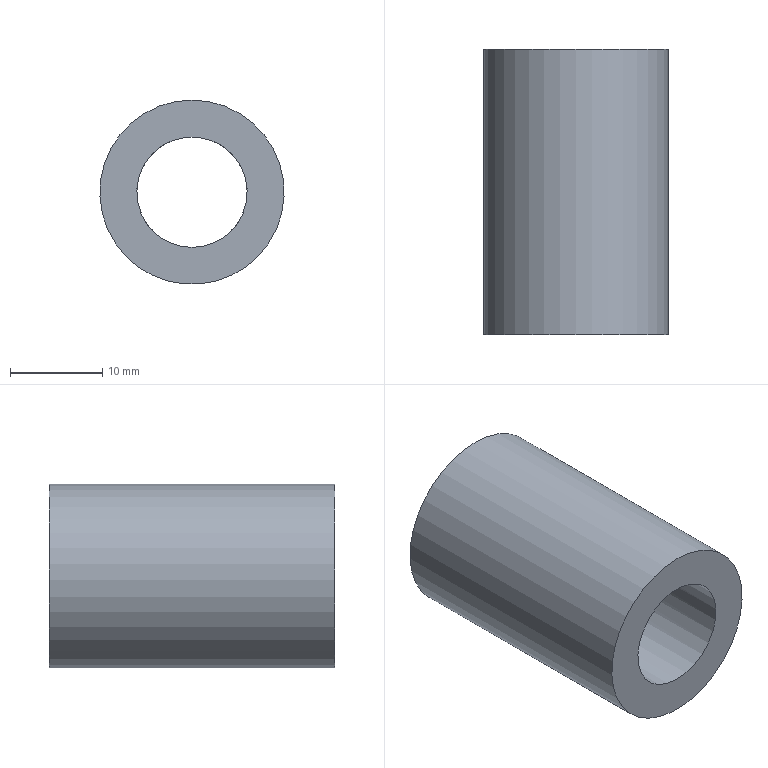Part | NX | features solid 2 | 1 solid | 4 faces | box 20 x 31 x 20 mm | volume 6233 mm3 | plane 2 | cylinder 2 | commonest cylinder face diameters 12 x1 20 x1
STEP:
#1=CARTESIAN_POINT('',(675.,144.,-20.));
#2=VERTEX_POINT('',#1);
#3=CARTESIAN_POINT('',(675.,144.,-30.));
#4=DIRECTION('',(0.,1.,0.));
#5=DIRECTION('',(0.,0.,1.));
#6=AXIS2_PLACEMENT_3D('',#3,#4,#5);
#7=CIRCLE('',#6,10.);
#8=EDGE_CURVE('',#2,#2,#7,.F.);
#9=ORIENTED_EDGE('',*,*,#8,.T.);
#10=EDGE_LOOP('',(#9));
#11=FACE_BOUND('',#10,.T.);
#12=CARTESIAN_POINT('',(675.,144.,-36.));
#13=VERTEX_POINT('',#12);
#14=CARTESIAN_POINT('',(675.,144.,-30.));
#15=DIRECTION('',(0.,-1.,0.));
#16=DIRECTION('',(0.,0.,-1.));
#17=AXIS2_PLACEMENT_3D('',#14,#15,#16);
#18=CIRCLE('',#17,6.);
#19=EDGE_CURVE('',#13,#13,#18,.T.);
#20=ORIENTED_EDGE('',*,*,#19,.F.);
#21=EDGE_LOOP('',(#20));
#22=FACE_BOUND('',#21,.T.);
#23=CARTESIAN_POINT('',(675.,144.,-30.));
#24=DIRECTION('',(0.,1.,0.));
#25=DIRECTION('',(0.,0.,1.));
#26=AXIS2_PLACEMENT_3D('',#23,#24,#25);
#27=PLANE('',#26);
#28=ADVANCED_FACE('',(#11,#22),#27,.F.);
#29=CARTESIAN_POINT('',(675.,175.,-20.));
#30=VERTEX_POINT('',#29);
#31=CARTESIAN_POINT('',(675.,175.,-30.));
#32=DIRECTION('',(0.,1.,0.));
#33=DIRECTION('',(0.,0.,1.));
#34=AXIS2_PLACEMENT_3D('',#31,#32,#33);
#35=CIRCLE('',#34,10.);
#36=EDGE_CURVE('',#30,#30,#35,.F.);
#37=ORIENTED_EDGE('',*,*,#36,.F.);
#38=EDGE_LOOP('',(#37));
#39=FACE_BOUND('',#38,.T.);
#40=CARTESIAN_POINT('',(675.,175.,-24.));
#41=VERTEX_POINT('',#40);
#42=CARTESIAN_POINT('',(675.,175.,-30.));
#43=DIRECTION('',(0.,1.,0.));
#44=DIRECTION('',(0.,0.,1.));
#45=AXIS2_PLACEMENT_3D('',#42,#43,#44);
#46=CIRCLE('',#45,6.);
#47=EDGE_CURVE('',#41,#41,#46,.F.);
#48=ORIENTED_EDGE('',*,*,#47,.T.);
#49=EDGE_LOOP('',(#48));
#50=FACE_BOUND('',#49,.T.);
#51=CARTESIAN_POINT('',(675.,175.,-30.));
#52=DIRECTION('',(0.,1.,0.));
#53=DIRECTION('',(0.,0.,1.));
#54=AXIS2_PLACEMENT_3D('',#51,#52,#53);
#55=PLANE('',#54);
#56=ADVANCED_FACE('',(#39,#50),#55,.T.);
#57=ORIENTED_EDGE('',*,*,#8,.F.);
#58=EDGE_LOOP('',(#57));
#59=FACE_BOUND('',#58,.T.);
#60=ORIENTED_EDGE('',*,*,#36,.T.);
#61=EDGE_LOOP('',(#60));
#62=FACE_BOUND('',#61,.T.);
#63=CARTESIAN_POINT('',(675.,174.,-30.));
#64=DIRECTION('',(0.,-1.,0.));
#65=DIRECTION('',(0.,0.,-1.));
#66=AXIS2_PLACEMENT_3D('',#63,#64,#65);
#67=CYLINDRICAL_SURFACE('',#66,10.);
#68=ADVANCED_FACE('',(#59,#62),#67,.T.);
#69=ORIENTED_EDGE('',*,*,#19,.T.);
#70=EDGE_LOOP('',(#69));
#71=FACE_BOUND('',#70,.T.);
#72=ORIENTED_EDGE('',*,*,#47,.F.);
#73=EDGE_LOOP('',(#72));
#74=FACE_BOUND('',#73,.T.);
#75=CARTESIAN_POINT('',(675.,174.,-30.));
#76=DIRECTION('',(0.,-1.,0.));
#77=DIRECTION('',(0.,0.,-1.));
#78=AXIS2_PLACEMENT_3D('',#75,#76,#77);
#79=CYLINDRICAL_SURFACE('',#78,6.);
#80=ADVANCED_FACE('',(#71,#74),#79,.F.);
#81=CLOSED_SHELL('',(#28,#56,#68,#80));
#82=MANIFOLD_SOLID_BREP('',#81);
#83=(LENGTH_UNIT()NAMED_UNIT(*)SI_UNIT(.MILLI.,.METRE.));
#84=UNCERTAINTY_MEASURE_WITH_UNIT(LENGTH_MEASURE(0.00001),#83,'','');
#85=(NAMED_UNIT(*)PLANE_ANGLE_UNIT()SI_UNIT($,.RADIAN.));
#86=(NAMED_UNIT(*)SI_UNIT($,.STERADIAN.)SOLID_ANGLE_UNIT());
#87=(GEOMETRIC_REPRESENTATION_CONTEXT(3)GLOBAL_UNCERTAINTY_ASSIGNED_CONTEXT((#84))GLOBAL_UNIT_ASSIGNED_CONTEXT((#83,#85,#86))REPRESENTATION_CONTEXT('',''));
#88=ADVANCED_BREP_SHAPE_REPRESENTATION('',(#82),#87);